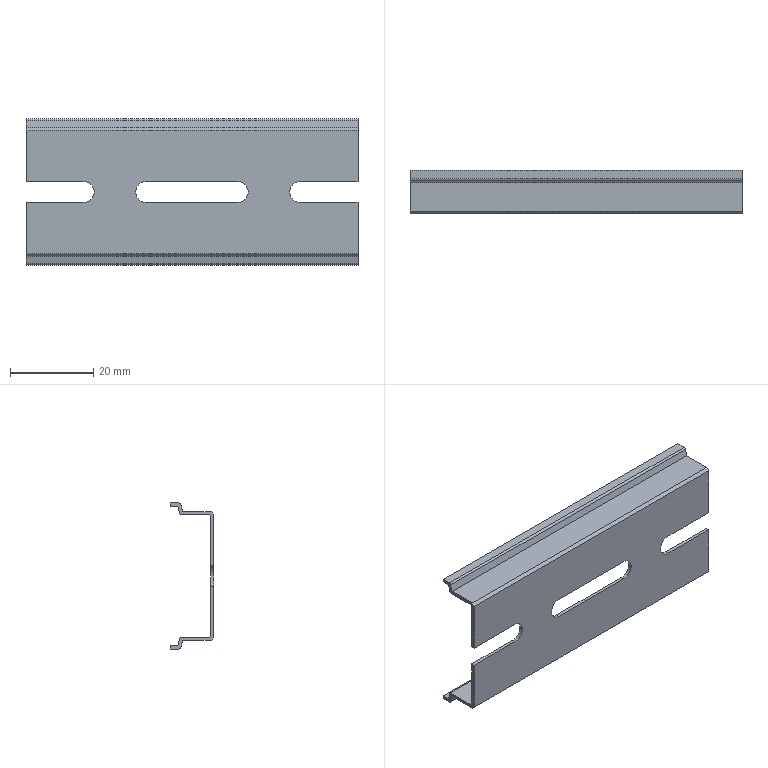Part | NX | 1 solid | 38 faces | box 79.8 x 10.5 x 35.1 mm | volume 3155 mm3 | plane 30 | cylinder 8 | commonest cylinder face diameters 5 x6 1 x2
STEP:
#1=CARTESIAN_POINT('',(44.9,-0.325,-0.15));
#2=VERTEX_POINT('',#1);
#3=CARTESIAN_POINT('',(44.9,-2.422,-0.15));
#4=VERTEX_POINT('',#3);
#5=CARTESIAN_POINT('',(44.9,0.,-0.15));
#6=DIRECTION('',(0.,-1.,0.));
#7=VECTOR('',#6,1000.);
#8=LINE('',#5,#7);
#9=EDGE_CURVE('',#2,#4,#8,.T.);
#10=ORIENTED_EDGE('',*,*,#9,.F.);
#11=CARTESIAN_POINT('',(-34.9,-0.325,-0.15));
#12=VERTEX_POINT('',#11);
#13=CARTESIAN_POINT('',(0.,-0.325,-0.15));
#14=DIRECTION('',(1.,0.,0.));
#15=VECTOR('',#14,1000.);
#16=LINE('',#13,#15);
#17=EDGE_CURVE('',#12,#2,#16,.T.);
#18=ORIENTED_EDGE('',*,*,#17,.F.);
#19=CARTESIAN_POINT('',(-34.9,-2.422,-0.15));
#20=VERTEX_POINT('',#19);
#21=CARTESIAN_POINT('',(-34.9,0.,-0.15));
#22=DIRECTION('',(0.,-1.,0.));
#23=VECTOR('',#22,1000.);
#24=LINE('',#21,#23);
#25=EDGE_CURVE('',#12,#20,#24,.T.);
#26=ORIENTED_EDGE('',*,*,#25,.T.);
#27=CARTESIAN_POINT('',(4.9,-2.422,-0.15));
#28=DIRECTION('',(-1.,0.,0.));
#29=VECTOR('',#28,1000.);
#30=LINE('',#27,#29);
#31=EDGE_CURVE('',#4,#20,#30,.T.);
#32=ORIENTED_EDGE('',*,*,#31,.F.);
#33=EDGE_LOOP('',(#10,#18,#26,#32));
#34=FACE_BOUND('',#33,.T.);
#35=CARTESIAN_POINT('',(4.9,-2.422,-0.15));
#36=DIRECTION('',(0.,0.,-1.));
#37=DIRECTION('',(0.,-1.,0.));
#38=AXIS2_PLACEMENT_3D('',#35,#36,#37);
#39=PLANE('',#38);
#40=ADVANCED_FACE('',(#34),#39,.F.);
#41=CARTESIAN_POINT('',(44.9,-10.169,-33.2));
#42=VERTEX_POINT('',#41);
#43=CARTESIAN_POINT('',(44.9,-3.325,-33.2));
#44=VERTEX_POINT('',#43);
#45=CARTESIAN_POINT('',(44.9,0.,-33.2));
#46=DIRECTION('',(0.,1.,0.));
#47=VECTOR('',#46,1000.);
#48=LINE('',#45,#47);
#49=EDGE_CURVE('',#42,#44,#48,.T.);
#50=ORIENTED_EDGE('',*,*,#49,.T.);
#51=CARTESIAN_POINT('',(44.9,-2.907,-34.871));
#52=VERTEX_POINT('',#51);
#53=CARTESIAN_POINT('',(44.9,-11.625,0.));
#54=DIRECTION('',(0.,0.2425,-0.9701));
#55=VECTOR('',#54,1000.);
#56=LINE('',#53,#55);
#57=EDGE_CURVE('',#44,#52,#56,.T.);
#58=ORIENTED_EDGE('',*,*,#57,.T.);
#59=CARTESIAN_POINT('',(44.9,-2.422,-35.25));
#60=VERTEX_POINT('',#59);
#61=CARTESIAN_POINT('',(44.9,-2.422,-34.75));
#62=DIRECTION('',(-1.,0.,0.));
#63=DIRECTION('',(0.,0.,1.));
#64=AXIS2_PLACEMENT_3D('',#61,#62,#63);
#65=CIRCLE('',#64,0.5);
#66=EDGE_CURVE('',#60,#52,#65,.T.);
#67=ORIENTED_EDGE('',*,*,#66,.F.);
#68=CARTESIAN_POINT('',(44.9,-0.325,-35.25));
#69=VERTEX_POINT('',#68);
#70=CARTESIAN_POINT('',(44.9,0.,-35.25));
#71=DIRECTION('',(0.,1.,0.));
#72=VECTOR('',#71,1000.);
#73=LINE('',#70,#72);
#74=EDGE_CURVE('',#60,#69,#73,.T.);
#75=ORIENTED_EDGE('',*,*,#74,.T.);
#76=CARTESIAN_POINT('',(44.9,-0.325,-34.45));
#77=VERTEX_POINT('',#76);
#78=CARTESIAN_POINT('',(44.9,-0.325,0.));
#79=DIRECTION('',(0.,0.,1.));
#80=VECTOR('',#79,1000.);
#81=LINE('',#78,#80);
#82=EDGE_CURVE('',#69,#77,#81,.T.);
#83=ORIENTED_EDGE('',*,*,#82,.T.);
#84=CARTESIAN_POINT('',(44.9,-2.188,-34.45));
#85=VERTEX_POINT('',#84);
#86=CARTESIAN_POINT('',(44.9,0.,-34.45));
#87=DIRECTION('',(0.,-1.,0.));
#88=VECTOR('',#87,1000.);
#89=LINE('',#86,#88);
#90=EDGE_CURVE('',#77,#85,#89,.T.);
#91=ORIENTED_EDGE('',*,*,#90,.T.);
#92=CARTESIAN_POINT('',(44.9,-2.7,-32.4));
#93=VERTEX_POINT('',#92);
#94=CARTESIAN_POINT('',(44.9,-10.8,0.));
#95=DIRECTION('',(0.,-0.2425,0.9701));
#96=VECTOR('',#95,1000.);
#97=LINE('',#94,#96);
#98=EDGE_CURVE('',#85,#93,#97,.T.);
#99=ORIENTED_EDGE('',*,*,#98,.T.);
#100=CARTESIAN_POINT('',(44.9,-9.834,-32.4));
#101=VERTEX_POINT('',#100);
#102=CARTESIAN_POINT('',(44.9,0.,-32.4));
#103=DIRECTION('',(0.,-1.,0.));
#104=VECTOR('',#103,1000.);
#105=LINE('',#102,#104);
#106=EDGE_CURVE('',#93,#101,#105,.T.);
#107=ORIENTED_EDGE('',*,*,#106,.T.);
#108=CARTESIAN_POINT('',(44.9,-10.025,-32.205));
#109=VERTEX_POINT('',#108);
#110=CARTESIAN_POINT('',(44.9,-41.673,0.));
#111=DIRECTION('',(0.,-0.7009,0.7133));
#112=VECTOR('',#111,1000.);
#113=LINE('',#110,#112);
#114=EDGE_CURVE('',#101,#109,#113,.T.);
#115=ORIENTED_EDGE('',*,*,#114,.T.);
#116=CARTESIAN_POINT('',(44.9,-10.025,-20.2));
#117=VERTEX_POINT('',#116);
#118=CARTESIAN_POINT('',(44.9,-10.025,0.));
#119=DIRECTION('',(0.,0.,1.));
#120=VECTOR('',#119,1000.);
#121=LINE('',#118,#120);
#122=EDGE_CURVE('',#109,#117,#121,.T.);
#123=ORIENTED_EDGE('',*,*,#122,.T.);
#124=CARTESIAN_POINT('',(44.9,-10.825,-20.2));
#125=VERTEX_POINT('',#124);
#126=CARTESIAN_POINT('',(44.9,0.,-20.2));
#127=DIRECTION('',(0.,-1.,0.));
#128=VECTOR('',#127,1000.);
#129=LINE('',#126,#128);
#130=EDGE_CURVE('',#117,#125,#129,.T.);
#131=ORIENTED_EDGE('',*,*,#130,.T.);
#132=CARTESIAN_POINT('',(44.9,-10.825,-32.532));
#133=VERTEX_POINT('',#132);
#134=CARTESIAN_POINT('',(44.9,-10.825,0.));
#135=DIRECTION('',(0.,0.,-1.));
#136=VECTOR('',#135,1000.);
#137=LINE('',#134,#136);
#138=EDGE_CURVE('',#125,#133,#137,.T.);
#139=ORIENTED_EDGE('',*,*,#138,.T.);
#140=CARTESIAN_POINT('',(44.9,-42.795,0.));
#141=DIRECTION('',(0.,0.7009,-0.7133));
#142=VECTOR('',#141,1000.);
#143=LINE('',#140,#142);
#144=EDGE_CURVE('',#133,#42,#143,.T.);
#145=ORIENTED_EDGE('',*,*,#144,.T.);
#146=EDGE_LOOP('',(#50,#58,#67,#75,#83,#91,#99,#107,#115,#123,#131,#139,#145));
#147=FACE_BOUND('',#146,.T.);
#148=CARTESIAN_POINT('',(44.9,-2.422,-0.65));
#149=DIRECTION('',(1.,0.,0.));
#150=DIRECTION('',(0.,0.,1.));
#151=AXIS2_PLACEMENT_3D('',#148,#149,#150);
#152=PLANE('',#151);
#153=ADVANCED_FACE('',(#147),#152,.T.);
#154=CARTESIAN_POINT('',(-34.9,-10.169,-33.2));
#155=VERTEX_POINT('',#154);
#156=CARTESIAN_POINT('',(-34.9,-3.325,-33.2));
#157=VERTEX_POINT('',#156);
#158=CARTESIAN_POINT('',(-34.9,0.,-33.2));
#159=DIRECTION('',(0.,1.,0.));
#160=VECTOR('',#159,1000.);
#161=LINE('',#158,#160);
#162=EDGE_CURVE('',#155,#157,#161,.T.);
#163=ORIENTED_EDGE('',*,*,#162,.T.);
#164=CARTESIAN_POINT('',(0.,-3.325,-33.2));
#165=DIRECTION('',(-1.,0.,0.));
#166=VECTOR('',#165,1000.);
#167=LINE('',#164,#166);
#168=EDGE_CURVE('',#44,#157,#167,.T.);
#169=ORIENTED_EDGE('',*,*,#168,.F.);
#170=ORIENTED_EDGE('',*,*,#49,.F.);
#171=CARTESIAN_POINT('',(0.,-10.169,-33.2));
#172=DIRECTION('',(-1.,0.,0.));
#173=VECTOR('',#172,1000.);
#174=LINE('',#171,#173);
#175=EDGE_CURVE('',#42,#155,#174,.T.);
#176=ORIENTED_EDGE('',*,*,#175,.T.);
#177=EDGE_LOOP('',(#163,#169,#170,#176));
#178=FACE_BOUND('',#177,.T.);
#179=CARTESIAN_POINT('',(4.9,-10.169,-33.2));
#180=DIRECTION('',(0.,0.,1.));
#181=DIRECTION('',(0.,-1.,0.));
#182=AXIS2_PLACEMENT_3D('',#179,#180,#181);
#183=PLANE('',#182);
#184=ADVANCED_FACE('',(#178),#183,.F.);
#185=ORIENTED_EDGE('',*,*,#138,.F.);
#186=CARTESIAN_POINT('',(31.,-10.825,-20.2));
#187=VERTEX_POINT('',#186);
#188=CARTESIAN_POINT('',(0.,-10.825,-20.2));
#189=DIRECTION('',(-1.,0.,0.));
#190=VECTOR('',#189,1000.);
#191=LINE('',#188,#190);
#192=EDGE_CURVE('',#125,#187,#191,.T.);
#193=ORIENTED_EDGE('',*,*,#192,.T.);
#194=CARTESIAN_POINT('',(28.5,-10.825,-17.7));
#195=VERTEX_POINT('',#194);
#196=CARTESIAN_POINT('',(31.,-10.825,-17.7));
#197=DIRECTION('',(0.,1.,0.));
#198=DIRECTION('',(-1.,0.,0.));
#199=AXIS2_PLACEMENT_3D('',#196,#197,#198);
#200=CIRCLE('',#199,2.5);
#201=EDGE_CURVE('',#187,#195,#200,.T.);
#202=ORIENTED_EDGE('',*,*,#201,.T.);
#203=CARTESIAN_POINT('',(31.,-10.825,-15.2));
#204=VERTEX_POINT('',#203);
#205=CARTESIAN_POINT('',(31.,-10.825,-17.7));
#206=DIRECTION('',(0.,1.,0.));
#207=DIRECTION('',(-1.,0.,0.));
#208=AXIS2_PLACEMENT_3D('',#205,#206,#207);
#209=CIRCLE('',#208,2.5);
#210=EDGE_CURVE('',#195,#204,#209,.T.);
#211=ORIENTED_EDGE('',*,*,#210,.T.);
#212=CARTESIAN_POINT('',(44.9,-10.825,-15.2));
#213=VERTEX_POINT('',#212);
#214=CARTESIAN_POINT('',(0.,-10.825,-15.2));
#215=DIRECTION('',(1.,0.,0.));
#216=VECTOR('',#215,1000.);
#217=LINE('',#214,#216);
#218=EDGE_CURVE('',#204,#213,#217,.T.);
#219=ORIENTED_EDGE('',*,*,#218,.T.);
#220=CARTESIAN_POINT('',(44.9,-10.825,-2.868));
#221=VERTEX_POINT('',#220);
#222=CARTESIAN_POINT('',(44.9,-10.825,0.));
#223=DIRECTION('',(0.,0.,-1.));
#224=VECTOR('',#223,1000.);
#225=LINE('',#222,#224);
#226=EDGE_CURVE('',#221,#213,#225,.T.);
#227=ORIENTED_EDGE('',*,*,#226,.F.);
#228=CARTESIAN_POINT('',(-34.9,-10.825,-2.868));
#229=VERTEX_POINT('',#228);
#230=CARTESIAN_POINT('',(0.,-10.825,-2.868));
#231=DIRECTION('',(1.,0.,0.));
#232=VECTOR('',#231,1000.);
#233=LINE('',#230,#232);
#234=EDGE_CURVE('',#229,#221,#233,.T.);
#235=ORIENTED_EDGE('',*,*,#234,.F.);
#236=CARTESIAN_POINT('',(-34.9,-10.825,-15.2));
#237=VERTEX_POINT('',#236);
#238=CARTESIAN_POINT('',(-34.9,-10.825,0.));
#239=DIRECTION('',(0.,0.,-1.));
#240=VECTOR('',#239,1000.);
#241=LINE('',#238,#240);
#242=EDGE_CURVE('',#229,#237,#241,.T.);
#243=ORIENTED_EDGE('',*,*,#242,.T.);
#244=CARTESIAN_POINT('',(-21.,-10.825,-15.2));
#245=VERTEX_POINT('',#244);
#246=CARTESIAN_POINT('',(0.,-10.825,-15.2));
#247=DIRECTION('',(1.,0.,0.));
#248=VECTOR('',#247,1000.);
#249=LINE('',#246,#248);
#250=EDGE_CURVE('',#237,#245,#249,.T.);
#251=ORIENTED_EDGE('',*,*,#250,.T.);
#252=CARTESIAN_POINT('',(-21.,-10.825,-20.2));
#253=VERTEX_POINT('',#252);
#254=CARTESIAN_POINT('',(-21.,-10.825,-17.7));
#255=DIRECTION('',(0.,1.,0.));
#256=DIRECTION('',(-1.,0.,0.));
#257=AXIS2_PLACEMENT_3D('',#254,#255,#256);
#258=CIRCLE('',#257,2.5);
#259=EDGE_CURVE('',#245,#253,#258,.T.);
#260=ORIENTED_EDGE('',*,*,#259,.T.);
#261=CARTESIAN_POINT('',(-34.9,-10.825,-20.2));
#262=VERTEX_POINT('',#261);
#263=CARTESIAN_POINT('',(0.,-10.825,-20.2));
#264=DIRECTION('',(-1.,0.,0.));
#265=VECTOR('',#264,1000.);
#266=LINE('',#263,#265);
#267=EDGE_CURVE('',#253,#262,#266,.T.);
#268=ORIENTED_EDGE('',*,*,#267,.T.);
#269=CARTESIAN_POINT('',(-34.9,-10.825,-32.532));
#270=VERTEX_POINT('',#269);
#271=CARTESIAN_POINT('',(-34.9,-10.825,0.));
#272=DIRECTION('',(0.,0.,-1.));
#273=VECTOR('',#272,1000.);
#274=LINE('',#271,#273);
#275=EDGE_CURVE('',#262,#270,#274,.T.);
#276=ORIENTED_EDGE('',*,*,#275,.T.);
#277=CARTESIAN_POINT('',(0.,-10.825,-32.532));
#278=DIRECTION('',(-1.,0.,0.));
#279=VECTOR('',#278,1000.);
#280=LINE('',#277,#279);
#281=EDGE_CURVE('',#133,#270,#280,.T.);
#282=ORIENTED_EDGE('',*,*,#281,.F.);
#283=EDGE_LOOP('',(#185,#193,#202,#211,#219,#227,#235,#243,#251,#260,#268,#276,#282));
#284=FACE_BOUND('',#283,.T.);
#285=CARTESIAN_POINT('',(16.,-10.825,-20.2));
#286=VERTEX_POINT('',#285);
#287=CARTESIAN_POINT('',(-6.,-10.825,-20.2));
#288=VERTEX_POINT('',#287);
#289=CARTESIAN_POINT('',(0.,-10.825,-20.2));
#290=DIRECTION('',(-1.,0.,0.));
#291=VECTOR('',#290,1000.);
#292=LINE('',#289,#291);
#293=EDGE_CURVE('',#286,#288,#292,.T.);
#294=ORIENTED_EDGE('',*,*,#293,.T.);
#295=CARTESIAN_POINT('',(-8.5,-10.825,-17.7));
#296=VERTEX_POINT('',#295);
#297=CARTESIAN_POINT('',(-6.,-10.825,-17.7));
#298=DIRECTION('',(0.,1.,0.));
#299=DIRECTION('',(-1.,0.,0.));
#300=AXIS2_PLACEMENT_3D('',#297,#298,#299);
#301=CIRCLE('',#300,2.5);
#302=EDGE_CURVE('',#288,#296,#301,.T.);
#303=ORIENTED_EDGE('',*,*,#302,.T.);
#304=CARTESIAN_POINT('',(-6.,-10.825,-15.2));
#305=VERTEX_POINT('',#304);
#306=CARTESIAN_POINT('',(-6.,-10.825,-17.7));
#307=DIRECTION('',(0.,1.,0.));
#308=DIRECTION('',(-1.,0.,0.));
#309=AXIS2_PLACEMENT_3D('',#306,#307,#308);
#310=CIRCLE('',#309,2.5);
#311=EDGE_CURVE('',#296,#305,#310,.T.);
#312=ORIENTED_EDGE('',*,*,#311,.T.);
#313=CARTESIAN_POINT('',(16.,-10.825,-15.2));
#314=VERTEX_POINT('',#313);
#315=CARTESIAN_POINT('',(0.,-10.825,-15.2));
#316=DIRECTION('',(1.,0.,0.));
#317=VECTOR('',#316,1000.);
#318=LINE('',#315,#317);
#319=EDGE_CURVE('',#305,#314,#318,.T.);
#320=ORIENTED_EDGE('',*,*,#319,.T.);
#321=CARTESIAN_POINT('',(16.,-10.825,-17.7));
#322=DIRECTION('',(0.,1.,0.));
#323=DIRECTION('',(-1.,0.,0.));
#324=AXIS2_PLACEMENT_3D('',#321,#322,#323);
#325=CIRCLE('',#324,2.5);
#326=EDGE_CURVE('',#314,#286,#325,.T.);
#327=ORIENTED_EDGE('',*,*,#326,.T.);
#328=EDGE_LOOP('',(#294,#303,#312,#320,#327));
#329=FACE_BOUND('',#328,.T.);
#330=CARTESIAN_POINT('',(4.9,-10.825,-2.868));
#331=DIRECTION('',(0.,1.,0.));
#332=DIRECTION('',(0.,0.,-1.));
#333=AXIS2_PLACEMENT_3D('',#330,#331,#332);
#334=PLANE('',#333);
#335=ADVANCED_FACE('',(#284,#329),#334,.F.);
#336=CARTESIAN_POINT('',(-34.9,-2.422,-35.25));
#337=VERTEX_POINT('',#336);
#338=CARTESIAN_POINT('',(-34.9,-2.907,-34.871));
#339=VERTEX_POINT('',#338);
#340=CARTESIAN_POINT('',(-34.9,-2.422,-34.75));
#341=DIRECTION('',(-1.,0.,0.));
#342=DIRECTION('',(0.,0.,1.));
#343=AXIS2_PLACEMENT_3D('',#340,#341,#342);
#344=CIRCLE('',#343,0.5);
#345=EDGE_CURVE('',#337,#339,#344,.T.);
#346=ORIENTED_EDGE('',*,*,#345,.F.);
#347=CARTESIAN_POINT('',(4.9,-2.422,-35.25));
#348=DIRECTION('',(1.,0.,0.));
#349=VECTOR('',#348,1000.);
#350=LINE('',#347,#349);
#351=EDGE_CURVE('',#337,#60,#350,.T.);
#352=ORIENTED_EDGE('',*,*,#351,.T.);
#353=ORIENTED_EDGE('',*,*,#66,.T.);
#354=CARTESIAN_POINT('',(4.9,-2.907,-34.871));
#355=DIRECTION('',(-1.,0.,0.));
#356=VECTOR('',#355,1000.);
#357=LINE('',#354,#356);
#358=EDGE_CURVE('',#52,#339,#357,.T.);
#359=ORIENTED_EDGE('',*,*,#358,.T.);
#360=EDGE_LOOP('',(#346,#352,#353,#359));
#361=FACE_BOUND('',#360,.T.);
#362=CARTESIAN_POINT('',(4.9,-2.422,-34.75));
#363=DIRECTION('',(-1.,0.,0.));
#364=DIRECTION('',(0.,0.,1.));
#365=AXIS2_PLACEMENT_3D('',#362,#363,#364);
#366=CYLINDRICAL_SURFACE('',#365,0.5);
#367=ADVANCED_FACE('',(#361),#366,.T.);
#368=CARTESIAN_POINT('',(-34.9,-0.325,-34.45));
#369=VERTEX_POINT('',#368);
#370=CARTESIAN_POINT('',(0.,-0.325,-34.45));
#371=DIRECTION('',(1.,0.,0.));
#372=VECTOR('',#371,1000.);
#373=LINE('',#370,#372);
#374=EDGE_CURVE('',#369,#77,#373,.T.);
#375=ORIENTED_EDGE('',*,*,#374,.T.);
#376=ORIENTED_EDGE('',*,*,#82,.F.);
#377=CARTESIAN_POINT('',(-34.9,-0.325,-35.25));
#378=VERTEX_POINT('',#377);
#379=CARTESIAN_POINT('',(0.,-0.325,-35.25));
#380=DIRECTION('',(1.,0.,0.));
#381=VECTOR('',#380,1000.);
#382=LINE('',#379,#381);
#383=EDGE_CURVE('',#378,#69,#382,.T.);
#384=ORIENTED_EDGE('',*,*,#383,.F.);
#385=CARTESIAN_POINT('',(-34.9,-0.325,0.));
#386=DIRECTION('',(0.,0.,1.));
#387=VECTOR('',#386,1000.);
#388=LINE('',#385,#387);
#389=EDGE_CURVE('',#378,#369,#388,.T.);
#390=ORIENTED_EDGE('',*,*,#389,.T.);
#391=EDGE_LOOP('',(#375,#376,#384,#390));
#392=FACE_BOUND('',#391,.T.);
#393=CARTESIAN_POINT('',(4.9,-0.325,-35.25));
#394=DIRECTION('',(0.,-1.,0.));
#395=DIRECTION('',(-1.,0.,0.));
#396=AXIS2_PLACEMENT_3D('',#393,#394,#395);
#397=PLANE('',#396);
#398=ADVANCED_FACE('',(#392),#397,.F.);
#399=CARTESIAN_POINT('',(-34.9,-3.325,-2.2));
#400=VERTEX_POINT('',#399);
#401=CARTESIAN_POINT('',(-34.9,-10.169,-2.2));
#402=VERTEX_POINT('',#401);
#403=CARTESIAN_POINT('',(-34.9,0.,-2.2));
#404=DIRECTION('',(0.,-1.,0.));
#405=VECTOR('',#404,1000.);
#406=LINE('',#403,#405);
#407=EDGE_CURVE('',#400,#402,#406,.T.);
#408=ORIENTED_EDGE('',*,*,#407,.T.);
#409=CARTESIAN_POINT('',(44.9,-10.169,-2.2));
#410=VERTEX_POINT('',#409);
#411=CARTESIAN_POINT('',(0.,-10.169,-2.2));
#412=DIRECTION('',(1.,0.,0.));
#413=VECTOR('',#412,1000.);
#414=LINE('',#411,#413);
#415=EDGE_CURVE('',#402,#410,#414,.T.);
#416=ORIENTED_EDGE('',*,*,#415,.T.);
#417=CARTESIAN_POINT('',(44.9,-3.325,-2.2));
#418=VERTEX_POINT('',#417);
#419=CARTESIAN_POINT('',(44.9,0.,-2.2));
#420=DIRECTION('',(0.,-1.,0.));
#421=VECTOR('',#420,1000.);
#422=LINE('',#419,#421);
#423=EDGE_CURVE('',#418,#410,#422,.T.);
#424=ORIENTED_EDGE('',*,*,#423,.F.);
#425=CARTESIAN_POINT('',(0.,-3.325,-2.2));
#426=DIRECTION('',(1.,0.,0.));
#427=VECTOR('',#426,1000.);
#428=LINE('',#425,#427);
#429=EDGE_CURVE('',#400,#418,#428,.T.);
#430=ORIENTED_EDGE('',*,*,#429,.F.);
#431=EDGE_LOOP('',(#408,#416,#424,#430));
#432=FACE_BOUND('',#431,.T.);
#433=CARTESIAN_POINT('',(4.9,-3.325,-2.2));
#434=DIRECTION('',(0.,0.,-1.));
#435=DIRECTION('',(-1.,0.,0.));
#436=AXIS2_PLACEMENT_3D('',#433,#434,#435);
#437=PLANE('',#436);
#438=ADVANCED_FACE('',(#432),#437,.F.);
#439=CARTESIAN_POINT('',(44.9,-0.325,-0.95));
#440=VERTEX_POINT('',#439);
#441=CARTESIAN_POINT('',(44.9,-0.325,0.));
#442=DIRECTION('',(0.,0.,1.));
#443=VECTOR('',#442,1000.);
#444=LINE('',#441,#443);
#445=EDGE_CURVE('',#440,#2,#444,.T.);
#446=ORIENTED_EDGE('',*,*,#445,.F.);
#447=CARTESIAN_POINT('',(-34.9,-0.325,-0.95));
#448=VERTEX_POINT('',#447);
#449=CARTESIAN_POINT('',(0.,-0.325,-0.95));
#450=DIRECTION('',(-1.,0.,0.));
#451=VECTOR('',#450,1000.);
#452=LINE('',#449,#451);
#453=EDGE_CURVE('',#440,#448,#452,.T.);
#454=ORIENTED_EDGE('',*,*,#453,.T.);
#455=CARTESIAN_POINT('',(-34.9,-0.325,0.));
#456=DIRECTION('',(0.,0.,1.));
#457=VECTOR('',#456,1000.);
#458=LINE('',#455,#457);
#459=EDGE_CURVE('',#448,#12,#458,.T.);
#460=ORIENTED_EDGE('',*,*,#459,.T.);
#461=ORIENTED_EDGE('',*,*,#17,.T.);
#462=EDGE_LOOP('',(#446,#454,#460,#461));
#463=FACE_BOUND('',#462,.T.);
#464=CARTESIAN_POINT('',(4.9,-0.325,-3.9));
#465=DIRECTION('',(0.,-1.,0.));
#466=DIRECTION('',(-1.,0.,0.));
#467=AXIS2_PLACEMENT_3D('',#464,#465,#466);
#468=PLANE('',#467);
#469=ADVANCED_FACE('',(#463),#468,.F.);
#470=CARTESIAN_POINT('',(-34.9,-2.907,-0.5287));
#471=VERTEX_POINT('',#470);
#472=CARTESIAN_POINT('',(-34.9,-2.422,-0.65));
#473=DIRECTION('',(-1.,0.,0.));
#474=DIRECTION('',(0.,0.,1.));
#475=AXIS2_PLACEMENT_3D('',#472,#473,#474);
#476=CIRCLE('',#475,0.5);
#477=EDGE_CURVE('',#471,#20,#476,.T.);
#478=ORIENTED_EDGE('',*,*,#477,.F.);
#479=CARTESIAN_POINT('',(44.9,-2.907,-0.5287));
#480=VERTEX_POINT('',#479);
#481=CARTESIAN_POINT('',(4.9,-2.907,-0.5287));
#482=DIRECTION('',(1.,0.,0.));
#483=VECTOR('',#482,1000.);
#484=LINE('',#481,#483);
#485=EDGE_CURVE('',#471,#480,#484,.T.);
#486=ORIENTED_EDGE('',*,*,#485,.T.);
#487=CARTESIAN_POINT('',(44.9,-2.422,-0.65));
#488=DIRECTION('',(-1.,0.,0.));
#489=DIRECTION('',(0.,0.,1.));
#490=AXIS2_PLACEMENT_3D('',#487,#488,#489);
#491=CIRCLE('',#490,0.5);
#492=EDGE_CURVE('',#480,#4,#491,.T.);
#493=ORIENTED_EDGE('',*,*,#492,.T.);
#494=ORIENTED_EDGE('',*,*,#31,.T.);
#495=EDGE_LOOP('',(#478,#486,#493,#494));
#496=FACE_BOUND('',#495,.T.);
#497=CARTESIAN_POINT('',(4.9,-2.422,-0.65));
#498=DIRECTION('',(-1.,0.,0.));
#499=DIRECTION('',(0.,0.,1.));
#500=AXIS2_PLACEMENT_3D('',#497,#498,#499);
#501=CYLINDRICAL_SURFACE('',#500,0.5);
#502=ADVANCED_FACE('',(#496),#501,.T.);
#503=ORIENTED_EDGE('',*,*,#162,.F.);
#504=CARTESIAN_POINT('',(-34.9,-42.795,0.));
#505=DIRECTION('',(0.,0.7009,-0.7133));
#506=VECTOR('',#505,1000.);
#507=LINE('',#504,#506);
#508=EDGE_CURVE('',#270,#155,#507,.T.);
#509=ORIENTED_EDGE('',*,*,#508,.F.);
#510=ORIENTED_EDGE('',*,*,#275,.F.);
#511=CARTESIAN_POINT('',(-34.9,-10.025,-20.2));
#512=VERTEX_POINT('',#511);
#513=CARTESIAN_POINT('',(-34.9,0.,-20.2));
#514=DIRECTION('',(0.,-1.,0.));
#515=VECTOR('',#514,1000.);
#516=LINE('',#513,#515);
#517=EDGE_CURVE('',#512,#262,#516,.T.);
#518=ORIENTED_EDGE('',*,*,#517,.F.);
#519=CARTESIAN_POINT('',(-34.9,-10.025,-32.205));
#520=VERTEX_POINT('',#519);
#521=CARTESIAN_POINT('',(-34.9,-10.025,0.));
#522=DIRECTION('',(0.,0.,1.));
#523=VECTOR('',#522,1000.);
#524=LINE('',#521,#523);
#525=EDGE_CURVE('',#520,#512,#524,.T.);
#526=ORIENTED_EDGE('',*,*,#525,.F.);
#527=CARTESIAN_POINT('',(-34.9,-9.834,-32.4));
#528=VERTEX_POINT('',#527);
#529=CARTESIAN_POINT('',(-34.9,-41.673,0.));
#530=DIRECTION('',(0.,-0.7009,0.7133));
#531=VECTOR('',#530,1000.);
#532=LINE('',#529,#531);
#533=EDGE_CURVE('',#528,#520,#532,.T.);
#534=ORIENTED_EDGE('',*,*,#533,.F.);
#535=CARTESIAN_POINT('',(-34.9,-2.7,-32.4));
#536=VERTEX_POINT('',#535);
#537=CARTESIAN_POINT('',(-34.9,0.,-32.4));
#538=DIRECTION('',(0.,-1.,0.));
#539=VECTOR('',#538,1000.);
#540=LINE('',#537,#539);
#541=EDGE_CURVE('',#536,#528,#540,.T.);
#542=ORIENTED_EDGE('',*,*,#541,.F.);
#543=CARTESIAN_POINT('',(-34.9,-2.188,-34.45));
#544=VERTEX_POINT('',#543);
#545=CARTESIAN_POINT('',(-34.9,-10.8,0.));
#546=DIRECTION('',(0.,-0.2425,0.9701));
#547=VECTOR('',#546,1000.);
#548=LINE('',#545,#547);
#549=EDGE_CURVE('',#544,#536,#548,.T.);
#550=ORIENTED_EDGE('',*,*,#549,.F.);
#551=CARTESIAN_POINT('',(-34.9,0.,-34.45));
#552=DIRECTION('',(0.,-1.,0.));
#553=VECTOR('',#552,1000.);
#554=LINE('',#551,#553);
#555=EDGE_CURVE('',#369,#544,#554,.T.);
#556=ORIENTED_EDGE('',*,*,#555,.F.);
#557=ORIENTED_EDGE('',*,*,#389,.F.);
#558=CARTESIAN_POINT('',(-34.9,0.,-35.25));
#559=DIRECTION('',(0.,1.,0.));
#560=VECTOR('',#559,1000.);
#561=LINE('',#558,#560);
#562=EDGE_CURVE('',#337,#378,#561,.T.);
#563=ORIENTED_EDGE('',*,*,#562,.F.);
#564=ORIENTED_EDGE('',*,*,#345,.T.);
#565=CARTESIAN_POINT('',(-34.9,-11.625,0.));
#566=DIRECTION('',(0.,0.2425,-0.9701));
#567=VECTOR('',#566,1000.);
#568=LINE('',#565,#567);
#569=EDGE_CURVE('',#157,#339,#568,.T.);
#570=ORIENTED_EDGE('',*,*,#569,.F.);
#571=EDGE_LOOP('',(#503,#509,#510,#518,#526,#534,#542,#550,#556,#557,#563,#564,#570));
#572=FACE_BOUND('',#571,.T.);
#573=CARTESIAN_POINT('',(-34.9,-2.422,-0.65));
#574=DIRECTION('',(1.,0.,0.));
#575=DIRECTION('',(0.,0.,1.));
#576=AXIS2_PLACEMENT_3D('',#573,#574,#575);
#577=PLANE('',#576);
#578=ADVANCED_FACE('',(#572),#577,.F.);
#579=CARTESIAN_POINT('',(44.9,-8.007,0.));
#580=DIRECTION('',(0.,-0.7009,-0.7133));
#581=VECTOR('',#580,1000.);
#582=LINE('',#579,#581);
#583=EDGE_CURVE('',#410,#221,#582,.T.);
#584=ORIENTED_EDGE('',*,*,#583,.F.);
#585=ORIENTED_EDGE('',*,*,#415,.F.);
#586=CARTESIAN_POINT('',(-34.9,-8.007,0.));
#587=DIRECTION('',(0.,-0.7009,-0.7133));
#588=VECTOR('',#587,1000.);
#589=LINE('',#586,#588);
#590=EDGE_CURVE('',#402,#229,#589,.T.);
#591=ORIENTED_EDGE('',*,*,#590,.T.);
#592=ORIENTED_EDGE('',*,*,#234,.T.);
#593=EDGE_LOOP('',(#584,#585,#591,#592));
#594=FACE_BOUND('',#593,.T.);
#595=CARTESIAN_POINT('',(4.9,-10.825,-2.868));
#596=DIRECTION('',(0.,0.7133,-0.7009));
#597=DIRECTION('',(-1.,0.,0.));
#598=AXIS2_PLACEMENT_3D('',#595,#596,#597);
#599=PLANE('',#598);
#600=ADVANCED_FACE('',(#594),#599,.F.);
#601=ORIENTED_EDGE('',*,*,#74,.F.);
#602=ORIENTED_EDGE('',*,*,#351,.F.);
#603=ORIENTED_EDGE('',*,*,#562,.T.);
#604=ORIENTED_EDGE('',*,*,#383,.T.);
#605=EDGE_LOOP('',(#601,#602,#603,#604));
#606=FACE_BOUND('',#605,.T.);
#607=CARTESIAN_POINT('',(4.9,-2.422,-35.25));
#608=DIRECTION('',(0.,0.,1.));
#609=DIRECTION('',(0.,-1.,0.));
#610=AXIS2_PLACEMENT_3D('',#607,#608,#609);
#611=PLANE('',#610);
#612=ADVANCED_FACE('',(#606),#611,.F.);
#613=ORIENTED_EDGE('',*,*,#144,.F.);
#614=ORIENTED_EDGE('',*,*,#281,.T.);
#615=ORIENTED_EDGE('',*,*,#508,.T.);
#616=ORIENTED_EDGE('',*,*,#175,.F.);
#617=EDGE_LOOP('',(#613,#614,#615,#616));
#618=FACE_BOUND('',#617,.T.);
#619=CARTESIAN_POINT('',(4.9,-10.825,-32.532));
#620=DIRECTION('',(0.,0.7133,0.7009));
#621=DIRECTION('',(1.,0.,0.));
#622=AXIS2_PLACEMENT_3D('',#619,#620,#621);
#623=PLANE('',#622);
#624=ADVANCED_FACE('',(#618),#623,.F.);
#625=ORIENTED_EDGE('',*,*,#57,.F.);
#626=ORIENTED_EDGE('',*,*,#168,.T.);
#627=ORIENTED_EDGE('',*,*,#569,.T.);
#628=ORIENTED_EDGE('',*,*,#358,.F.);
#629=EDGE_LOOP('',(#625,#626,#627,#628));
#630=FACE_BOUND('',#629,.T.);
#631=CARTESIAN_POINT('',(4.9,-2.907,-34.871));
#632=DIRECTION('',(0.,0.9701,0.2425));
#633=DIRECTION('',(1.,0.,0.));
#634=AXIS2_PLACEMENT_3D('',#631,#632,#633);
#635=PLANE('',#634);
#636=ADVANCED_FACE('',(#630),#635,.F.);
#637=CARTESIAN_POINT('',(44.9,-2.775,0.));
#638=DIRECTION('',(0.,-0.2425,-0.9701));
#639=VECTOR('',#638,1000.);
#640=LINE('',#637,#639);
#641=EDGE_CURVE('',#480,#418,#640,.T.);
#642=ORIENTED_EDGE('',*,*,#641,.F.);
#643=ORIENTED_EDGE('',*,*,#485,.F.);
#644=CARTESIAN_POINT('',(-34.9,-2.775,0.));
#645=DIRECTION('',(0.,-0.2425,-0.9701));
#646=VECTOR('',#645,1000.);
#647=LINE('',#644,#646);
#648=EDGE_CURVE('',#471,#400,#647,.T.);
#649=ORIENTED_EDGE('',*,*,#648,.T.);
#650=ORIENTED_EDGE('',*,*,#429,.T.);
#651=EDGE_LOOP('',(#642,#643,#649,#650));
#652=FACE_BOUND('',#651,.T.);
#653=CARTESIAN_POINT('',(4.9,-2.907,-0.5287));
#654=DIRECTION('',(0.,0.9701,-0.2425));
#655=DIRECTION('',(-1.,0.,0.));
#656=AXIS2_PLACEMENT_3D('',#653,#654,#655);
#657=PLANE('',#656);
#658=ADVANCED_FACE('',(#652),#657,.F.);
#659=ORIENTED_EDGE('',*,*,#549,.T.);
#660=CARTESIAN_POINT('',(0.,-2.7,-32.4));
#661=DIRECTION('',(-1.,0.,0.));
#662=VECTOR('',#661,1000.);
#663=LINE('',#660,#662);
#664=EDGE_CURVE('',#93,#536,#663,.T.);
#665=ORIENTED_EDGE('',*,*,#664,.F.);
#666=ORIENTED_EDGE('',*,*,#98,.F.);
#667=CARTESIAN_POINT('',(0.,-2.188,-34.45));
#668=DIRECTION('',(-1.,0.,0.));
#669=VECTOR('',#668,1000.);
#670=LINE('',#667,#669);
#671=EDGE_CURVE('',#85,#544,#670,.T.);
#672=ORIENTED_EDGE('',*,*,#671,.T.);
#673=EDGE_LOOP('',(#659,#665,#666,#672));
#674=FACE_BOUND('',#673,.T.);
#675=CARTESIAN_POINT('',(5.88,-2.7,-32.4));
#676=DIRECTION('',(0.,-0.9701,-0.2425));
#677=DIRECTION('',(0.,0.2425,-0.9701));
#678=AXIS2_PLACEMENT_3D('',#675,#676,#677);
#679=PLANE('',#678);
#680=ADVANCED_FACE('',(#674),#679,.F.);
#681=ORIENTED_EDGE('',*,*,#106,.F.);
#682=ORIENTED_EDGE('',*,*,#664,.T.);
#683=ORIENTED_EDGE('',*,*,#541,.T.);
#684=CARTESIAN_POINT('',(0.,-9.834,-32.4));
#685=DIRECTION('',(-1.,0.,0.));
#686=VECTOR('',#685,1000.);
#687=LINE('',#684,#686);
#688=EDGE_CURVE('',#101,#528,#687,.T.);
#689=ORIENTED_EDGE('',*,*,#688,.F.);
#690=EDGE_LOOP('',(#681,#682,#683,#689));
#691=FACE_BOUND('',#690,.T.);
#692=CARTESIAN_POINT('',(5.88,-9.834,-32.4));
#693=DIRECTION('',(0.,0.,-1.));
#694=DIRECTION('',(0.,-1.,0.));
#695=AXIS2_PLACEMENT_3D('',#692,#693,#694);
#696=PLANE('',#695);
#697=ADVANCED_FACE('',(#691),#696,.F.);
#698=ORIENTED_EDGE('',*,*,#114,.F.);
#699=ORIENTED_EDGE('',*,*,#688,.T.);
#700=ORIENTED_EDGE('',*,*,#533,.T.);
#701=CARTESIAN_POINT('',(0.,-10.025,-32.205));
#702=DIRECTION('',(-1.,0.,0.));
#703=VECTOR('',#702,1000.);
#704=LINE('',#701,#703);
#705=EDGE_CURVE('',#109,#520,#704,.T.);
#706=ORIENTED_EDGE('',*,*,#705,.F.);
#707=EDGE_LOOP('',(#698,#699,#700,#706));
#708=FACE_BOUND('',#707,.T.);
#709=CARTESIAN_POINT('',(5.88,-10.025,-32.205));
#710=DIRECTION('',(0.,-0.7133,-0.7009));
#711=DIRECTION('',(0.,0.7009,-0.7133));
#712=AXIS2_PLACEMENT_3D('',#709,#710,#711);
#713=PLANE('',#712);
#714=ADVANCED_FACE('',(#708),#713,.F.);
#715=CARTESIAN_POINT('',(-34.9,-10.025,-15.2));
#716=VERTEX_POINT('',#715);
#717=CARTESIAN_POINT('',(-34.9,-10.025,-3.195));
#718=VERTEX_POINT('',#717);
#719=CARTESIAN_POINT('',(-34.9,-10.025,0.));
#720=DIRECTION('',(0.,0.,1.));
#721=VECTOR('',#720,1000.);
#722=LINE('',#719,#721);
#723=EDGE_CURVE('',#716,#718,#722,.T.);
#724=ORIENTED_EDGE('',*,*,#723,.T.);
#725=CARTESIAN_POINT('',(44.9,-10.025,-3.195));
#726=VERTEX_POINT('',#725);
#727=CARTESIAN_POINT('',(0.,-10.025,-3.195));
#728=DIRECTION('',(-1.,0.,0.));
#729=VECTOR('',#728,1000.);
#730=LINE('',#727,#729);
#731=EDGE_CURVE('',#726,#718,#730,.T.);
#732=ORIENTED_EDGE('',*,*,#731,.F.);
#733=CARTESIAN_POINT('',(44.9,-10.025,-15.2));
#734=VERTEX_POINT('',#733);
#735=CARTESIAN_POINT('',(44.9,-10.025,0.));
#736=DIRECTION('',(0.,0.,1.));
#737=VECTOR('',#736,1000.);
#738=LINE('',#735,#737);
#739=EDGE_CURVE('',#734,#726,#738,.T.);
#740=ORIENTED_EDGE('',*,*,#739,.F.);
#741=CARTESIAN_POINT('',(31.,-10.025,-15.2));
#742=VERTEX_POINT('',#741);
#743=CARTESIAN_POINT('',(0.,-10.025,-15.2));
#744=DIRECTION('',(-1.,0.,0.));
#745=VECTOR('',#744,1000.);
#746=LINE('',#743,#745);
#747=EDGE_CURVE('',#734,#742,#746,.T.);
#748=ORIENTED_EDGE('',*,*,#747,.T.);
#749=CARTESIAN_POINT('',(28.5,-10.025,-17.7));
#750=VERTEX_POINT('',#749);
#751=CARTESIAN_POINT('',(31.,-10.025,-17.7));
#752=DIRECTION('',(0.,1.,0.));
#753=DIRECTION('',(-1.,0.,0.));
#754=AXIS2_PLACEMENT_3D('',#751,#752,#753);
#755=CIRCLE('',#754,2.5);
#756=EDGE_CURVE('',#750,#742,#755,.T.);
#757=ORIENTED_EDGE('',*,*,#756,.F.);
#758=CARTESIAN_POINT('',(31.,-10.025,-20.2));
#759=VERTEX_POINT('',#758);
#760=CARTESIAN_POINT('',(31.,-10.025,-17.7));
#761=DIRECTION('',(0.,1.,0.));
#762=DIRECTION('',(-1.,0.,0.));
#763=AXIS2_PLACEMENT_3D('',#760,#761,#762);
#764=CIRCLE('',#763,2.5);
#765=EDGE_CURVE('',#759,#750,#764,.T.);
#766=ORIENTED_EDGE('',*,*,#765,.F.);
#767=CARTESIAN_POINT('',(0.,-10.025,-20.2));
#768=DIRECTION('',(1.,0.,0.));
#769=VECTOR('',#768,1000.);
#770=LINE('',#767,#769);
#771=EDGE_CURVE('',#759,#117,#770,.T.);
#772=ORIENTED_EDGE('',*,*,#771,.T.);
#773=ORIENTED_EDGE('',*,*,#122,.F.);
#774=ORIENTED_EDGE('',*,*,#705,.T.);
#775=ORIENTED_EDGE('',*,*,#525,.T.);
#776=CARTESIAN_POINT('',(-21.,-10.025,-20.2));
#777=VERTEX_POINT('',#776);
#778=CARTESIAN_POINT('',(0.,-10.025,-20.2));
#779=DIRECTION('',(1.,0.,0.));
#780=VECTOR('',#779,1000.);
#781=LINE('',#778,#780);
#782=EDGE_CURVE('',#512,#777,#781,.T.);
#783=ORIENTED_EDGE('',*,*,#782,.T.);
#784=CARTESIAN_POINT('',(-21.,-10.025,-15.2));
#785=VERTEX_POINT('',#784);
#786=CARTESIAN_POINT('',(-21.,-10.025,-17.7));
#787=DIRECTION('',(0.,1.,0.));
#788=DIRECTION('',(-1.,0.,0.));
#789=AXIS2_PLACEMENT_3D('',#786,#787,#788);
#790=CIRCLE('',#789,2.5);
#791=EDGE_CURVE('',#785,#777,#790,.T.);
#792=ORIENTED_EDGE('',*,*,#791,.F.);
#793=CARTESIAN_POINT('',(0.,-10.025,-15.2));
#794=DIRECTION('',(-1.,0.,0.));
#795=VECTOR('',#794,1000.);
#796=LINE('',#793,#795);
#797=EDGE_CURVE('',#785,#716,#796,.T.);
#798=ORIENTED_EDGE('',*,*,#797,.T.);
#799=EDGE_LOOP('',(#724,#732,#740,#748,#757,#766,#772,#773,#774,#775,#783,#792,#798));
#800=FACE_BOUND('',#799,.T.);
#801=CARTESIAN_POINT('',(16.,-10.025,-15.2));
#802=VERTEX_POINT('',#801);
#803=CARTESIAN_POINT('',(-6.,-10.025,-15.2));
#804=VERTEX_POINT('',#803);
#805=CARTESIAN_POINT('',(0.,-10.025,-15.2));
#806=DIRECTION('',(-1.,0.,0.));
#807=VECTOR('',#806,1000.);
#808=LINE('',#805,#807);
#809=EDGE_CURVE('',#802,#804,#808,.T.);
#810=ORIENTED_EDGE('',*,*,#809,.T.);
#811=CARTESIAN_POINT('',(-8.5,-10.025,-17.7));
#812=VERTEX_POINT('',#811);
#813=CARTESIAN_POINT('',(-6.,-10.025,-17.7));
#814=DIRECTION('',(0.,1.,0.));
#815=DIRECTION('',(-1.,0.,0.));
#816=AXIS2_PLACEMENT_3D('',#813,#814,#815);
#817=CIRCLE('',#816,2.5);
#818=EDGE_CURVE('',#812,#804,#817,.T.);
#819=ORIENTED_EDGE('',*,*,#818,.F.);
#820=CARTESIAN_POINT('',(-6.,-10.025,-20.2));
#821=VERTEX_POINT('',#820);
#822=CARTESIAN_POINT('',(-6.,-10.025,-17.7));
#823=DIRECTION('',(0.,1.,0.));
#824=DIRECTION('',(-1.,0.,0.));
#825=AXIS2_PLACEMENT_3D('',#822,#823,#824);
#826=CIRCLE('',#825,2.5);
#827=EDGE_CURVE('',#821,#812,#826,.T.);
#828=ORIENTED_EDGE('',*,*,#827,.F.);
#829=CARTESIAN_POINT('',(16.,-10.025,-20.2));
#830=VERTEX_POINT('',#829);
#831=CARTESIAN_POINT('',(0.,-10.025,-20.2));
#832=DIRECTION('',(1.,0.,0.));
#833=VECTOR('',#832,1000.);
#834=LINE('',#831,#833);
#835=EDGE_CURVE('',#821,#830,#834,.T.);
#836=ORIENTED_EDGE('',*,*,#835,.T.);
#837=CARTESIAN_POINT('',(16.,-10.025,-17.7));
#838=DIRECTION('',(0.,1.,0.));
#839=DIRECTION('',(-1.,0.,0.));
#840=AXIS2_PLACEMENT_3D('',#837,#838,#839);
#841=CIRCLE('',#840,2.5);
#842=EDGE_CURVE('',#802,#830,#841,.T.);
#843=ORIENTED_EDGE('',*,*,#842,.F.);
#844=EDGE_LOOP('',(#810,#819,#828,#836,#843));
#845=FACE_BOUND('',#844,.T.);
#846=CARTESIAN_POINT('',(5.88,-10.025,-3.195));
#847=DIRECTION('',(0.,-1.,0.));
#848=DIRECTION('',(-1.,0.,0.));
#849=AXIS2_PLACEMENT_3D('',#846,#847,#848);
#850=PLANE('',#849);
#851=ADVANCED_FACE('',(#800,#845),#850,.F.);
#852=CARTESIAN_POINT('',(44.9,-9.834,-3.));
#853=VERTEX_POINT('',#852);
#854=CARTESIAN_POINT('',(44.9,-6.885,0.));
#855=DIRECTION('',(0.,0.7009,0.7133));
#856=VECTOR('',#855,1000.);
#857=LINE('',#854,#856);
#858=EDGE_CURVE('',#726,#853,#857,.T.);
#859=ORIENTED_EDGE('',*,*,#858,.F.);
#860=ORIENTED_EDGE('',*,*,#731,.T.);
#861=CARTESIAN_POINT('',(-34.9,-9.834,-3.));
#862=VERTEX_POINT('',#861);
#863=CARTESIAN_POINT('',(-34.9,-6.885,0.));
#864=DIRECTION('',(0.,0.7009,0.7133));
#865=VECTOR('',#864,1000.);
#866=LINE('',#863,#865);
#867=EDGE_CURVE('',#718,#862,#866,.T.);
#868=ORIENTED_EDGE('',*,*,#867,.T.);
#869=CARTESIAN_POINT('',(0.,-9.834,-3.));
#870=DIRECTION('',(-1.,0.,0.));
#871=VECTOR('',#870,1000.);
#872=LINE('',#869,#871);
#873=EDGE_CURVE('',#853,#862,#872,.T.);
#874=ORIENTED_EDGE('',*,*,#873,.F.);
#875=EDGE_LOOP('',(#859,#860,#868,#874));
#876=FACE_BOUND('',#875,.T.);
#877=CARTESIAN_POINT('',(5.88,-9.834,-3.));
#878=DIRECTION('',(0.,-0.7133,0.7009));
#879=DIRECTION('',(-1.,0.,0.));
#880=AXIS2_PLACEMENT_3D('',#877,#878,#879);
#881=PLANE('',#880);
#882=ADVANCED_FACE('',(#876),#881,.F.);
#883=CARTESIAN_POINT('',(-34.9,-2.7,-3.));
#884=VERTEX_POINT('',#883);
#885=CARTESIAN_POINT('',(-34.9,0.,-3.));
#886=DIRECTION('',(0.,1.,0.));
#887=VECTOR('',#886,1000.);
#888=LINE('',#885,#887);
#889=EDGE_CURVE('',#862,#884,#888,.T.);
#890=ORIENTED_EDGE('',*,*,#889,.T.);
#891=CARTESIAN_POINT('',(44.9,-2.7,-3.));
#892=VERTEX_POINT('',#891);
#893=CARTESIAN_POINT('',(0.,-2.7,-3.));
#894=DIRECTION('',(-1.,0.,0.));
#895=VECTOR('',#894,1000.);
#896=LINE('',#893,#895);
#897=EDGE_CURVE('',#892,#884,#896,.T.);
#898=ORIENTED_EDGE('',*,*,#897,.F.);
#899=CARTESIAN_POINT('',(44.9,0.,-3.));
#900=DIRECTION('',(0.,1.,0.));
#901=VECTOR('',#900,1000.);
#902=LINE('',#899,#901);
#903=EDGE_CURVE('',#853,#892,#902,.T.);
#904=ORIENTED_EDGE('',*,*,#903,.F.);
#905=ORIENTED_EDGE('',*,*,#873,.T.);
#906=EDGE_LOOP('',(#890,#898,#904,#905));
#907=FACE_BOUND('',#906,.T.);
#908=CARTESIAN_POINT('',(5.88,-2.7,-3.));
#909=DIRECTION('',(0.,0.,1.));
#910=DIRECTION('',(0.,-1.,0.));
#911=AXIS2_PLACEMENT_3D('',#908,#909,#910);
#912=PLANE('',#911);
#913=ADVANCED_FACE('',(#907),#912,.F.);
#914=CARTESIAN_POINT('',(44.9,-2.188,-0.95));
#915=VERTEX_POINT('',#914);
#916=CARTESIAN_POINT('',(44.9,-1.95,0.));
#917=DIRECTION('',(0.,0.2425,0.9701));
#918=VECTOR('',#917,1000.);
#919=LINE('',#916,#918);
#920=EDGE_CURVE('',#892,#915,#919,.T.);
#921=ORIENTED_EDGE('',*,*,#920,.F.);
#922=ORIENTED_EDGE('',*,*,#897,.T.);
#923=CARTESIAN_POINT('',(-34.9,-2.188,-0.95));
#924=VERTEX_POINT('',#923);
#925=CARTESIAN_POINT('',(-34.9,-1.95,0.));
#926=DIRECTION('',(0.,0.2425,0.9701));
#927=VECTOR('',#926,1000.);
#928=LINE('',#925,#927);
#929=EDGE_CURVE('',#884,#924,#928,.T.);
#930=ORIENTED_EDGE('',*,*,#929,.T.);
#931=CARTESIAN_POINT('',(0.,-2.188,-0.95));
#932=DIRECTION('',(-1.,0.,0.));
#933=VECTOR('',#932,1000.);
#934=LINE('',#931,#933);
#935=EDGE_CURVE('',#915,#924,#934,.T.);
#936=ORIENTED_EDGE('',*,*,#935,.F.);
#937=EDGE_LOOP('',(#921,#922,#930,#936));
#938=FACE_BOUND('',#937,.T.);
#939=CARTESIAN_POINT('',(5.88,-2.188,-0.95));
#940=DIRECTION('',(0.,-0.9701,0.2425));
#941=DIRECTION('',(-1.,0.,0.));
#942=AXIS2_PLACEMENT_3D('',#939,#940,#941);
#943=PLANE('',#942);
#944=ADVANCED_FACE('',(#938),#943,.F.);
#945=CARTESIAN_POINT('',(44.9,0.,-0.95));
#946=DIRECTION('',(0.,1.,0.));
#947=VECTOR('',#946,1000.);
#948=LINE('',#945,#947);
#949=EDGE_CURVE('',#915,#440,#948,.T.);
#950=ORIENTED_EDGE('',*,*,#949,.F.);
#951=ORIENTED_EDGE('',*,*,#935,.T.);
#952=CARTESIAN_POINT('',(-34.9,0.,-0.95));
#953=DIRECTION('',(0.,1.,0.));
#954=VECTOR('',#953,1000.);
#955=LINE('',#952,#954);
#956=EDGE_CURVE('',#924,#448,#955,.T.);
#957=ORIENTED_EDGE('',*,*,#956,.T.);
#958=ORIENTED_EDGE('',*,*,#453,.F.);
#959=EDGE_LOOP('',(#950,#951,#957,#958));
#960=FACE_BOUND('',#959,.T.);
#961=CARTESIAN_POINT('',(5.88,-0.325,-0.95));
#962=DIRECTION('',(0.,0.,1.));
#963=DIRECTION('',(0.,-1.,0.));
#964=AXIS2_PLACEMENT_3D('',#961,#962,#963);
#965=PLANE('',#964);
#966=ADVANCED_FACE('',(#960),#965,.F.);
#967=ORIENTED_EDGE('',*,*,#555,.T.);
#968=ORIENTED_EDGE('',*,*,#671,.F.);
#969=ORIENTED_EDGE('',*,*,#90,.F.);
#970=ORIENTED_EDGE('',*,*,#374,.F.);
#971=EDGE_LOOP('',(#967,#968,#969,#970));
#972=FACE_BOUND('',#971,.T.);
#973=CARTESIAN_POINT('',(5.88,-2.188,-34.45));
#974=DIRECTION('',(0.,0.,-1.));
#975=DIRECTION('',(0.,-1.,0.));
#976=AXIS2_PLACEMENT_3D('',#973,#974,#975);
#977=PLANE('',#976);
#978=ADVANCED_FACE('',(#972),#977,.F.);
#979=CARTESIAN_POINT('',(-34.9,0.,-15.2));
#980=DIRECTION('',(0.,1.,0.));
#981=VECTOR('',#980,1000.);
#982=LINE('',#979,#981);
#983=EDGE_CURVE('',#237,#716,#982,.T.);
#984=ORIENTED_EDGE('',*,*,#983,.F.);
#985=ORIENTED_EDGE('',*,*,#242,.F.);
#986=ORIENTED_EDGE('',*,*,#590,.F.);
#987=ORIENTED_EDGE('',*,*,#407,.F.);
#988=ORIENTED_EDGE('',*,*,#648,.F.);
#989=ORIENTED_EDGE('',*,*,#477,.T.);
#990=ORIENTED_EDGE('',*,*,#25,.F.);
#991=ORIENTED_EDGE('',*,*,#459,.F.);
#992=ORIENTED_EDGE('',*,*,#956,.F.);
#993=ORIENTED_EDGE('',*,*,#929,.F.);
#994=ORIENTED_EDGE('',*,*,#889,.F.);
#995=ORIENTED_EDGE('',*,*,#867,.F.);
#996=ORIENTED_EDGE('',*,*,#723,.F.);
#997=EDGE_LOOP('',(#984,#985,#986,#987,#988,#989,#990,#991,#992,#993,#994,#995,#996));
#998=FACE_BOUND('',#997,.T.);
#999=CARTESIAN_POINT('',(-34.9,-2.422,-0.65));
#1000=DIRECTION('',(1.,0.,0.));
#1001=DIRECTION('',(0.,0.,1.));
#1002=AXIS2_PLACEMENT_3D('',#999,#1000,#1001);
#1003=PLANE('',#1002);
#1004=ADVANCED_FACE('',(#998),#1003,.F.);
#1005=CARTESIAN_POINT('',(44.9,0.,-15.2));
#1006=DIRECTION('',(0.,1.,0.));
#1007=VECTOR('',#1006,1000.);
#1008=LINE('',#1005,#1007);
#1009=EDGE_CURVE('',#213,#734,#1008,.T.);
#1010=ORIENTED_EDGE('',*,*,#1009,.T.);
#1011=ORIENTED_EDGE('',*,*,#739,.T.);
#1012=ORIENTED_EDGE('',*,*,#858,.T.);
#1013=ORIENTED_EDGE('',*,*,#903,.T.);
#1014=ORIENTED_EDGE('',*,*,#920,.T.);
#1015=ORIENTED_EDGE('',*,*,#949,.T.);
#1016=ORIENTED_EDGE('',*,*,#445,.T.);
#1017=ORIENTED_EDGE('',*,*,#9,.T.);
#1018=ORIENTED_EDGE('',*,*,#492,.F.);
#1019=ORIENTED_EDGE('',*,*,#641,.T.);
#1020=ORIENTED_EDGE('',*,*,#423,.T.);
#1021=ORIENTED_EDGE('',*,*,#583,.T.);
#1022=ORIENTED_EDGE('',*,*,#226,.T.);
#1023=EDGE_LOOP('',(#1010,#1011,#1012,#1013,#1014,#1015,#1016,#1017,#1018,#1019,#1020,#1021,#1022));
#1024=FACE_BOUND('',#1023,.T.);
#1025=CARTESIAN_POINT('',(44.9,-2.422,-0.65));
#1026=DIRECTION('',(1.,0.,0.));
#1027=DIRECTION('',(0.,0.,1.));
#1028=AXIS2_PLACEMENT_3D('',#1025,#1026,#1027);
#1029=PLANE('',#1028);
#1030=ADVANCED_FACE('',(#1024),#1029,.T.);
#1031=ORIENTED_EDGE('',*,*,#250,.F.);
#1032=ORIENTED_EDGE('',*,*,#983,.T.);
#1033=ORIENTED_EDGE('',*,*,#797,.F.);
#1034=CARTESIAN_POINT('',(-21.,-11.875,-15.2));
#1035=DIRECTION('',(0.,1.,0.));
#1036=VECTOR('',#1035,1000.);
#1037=LINE('',#1034,#1036);
#1038=EDGE_CURVE('',#245,#785,#1037,.T.);
#1039=ORIENTED_EDGE('',*,*,#1038,.F.);
#1040=EDGE_LOOP('',(#1031,#1032,#1033,#1039));
#1041=FACE_BOUND('',#1040,.T.);
#1042=CARTESIAN_POINT('',(-21.,-11.875,-15.2));
#1043=DIRECTION('',(0.,0.,1.));
#1044=DIRECTION('',(0.,-1.,0.));
#1045=AXIS2_PLACEMENT_3D('',#1042,#1043,#1044);
#1046=PLANE('',#1045);
#1047=ADVANCED_FACE('',(#1041),#1046,.F.);
#1048=CARTESIAN_POINT('',(28.5,-11.875,-17.7));
#1049=DIRECTION('',(0.,1.,0.));
#1050=VECTOR('',#1049,1000.);
#1051=LINE('',#1048,#1050);
#1052=EDGE_CURVE('',#195,#750,#1051,.T.);
#1053=ORIENTED_EDGE('',*,*,#1052,.F.);
#1054=ORIENTED_EDGE('',*,*,#201,.F.);
#1055=CARTESIAN_POINT('',(31.,-11.875,-20.2));
#1056=DIRECTION('',(0.,1.,0.));
#1057=VECTOR('',#1056,1000.);
#1058=LINE('',#1055,#1057);
#1059=EDGE_CURVE('',#187,#759,#1058,.T.);
#1060=ORIENTED_EDGE('',*,*,#1059,.T.);
#1061=ORIENTED_EDGE('',*,*,#765,.T.);
#1062=EDGE_LOOP('',(#1053,#1054,#1060,#1061));
#1063=FACE_BOUND('',#1062,.T.);
#1064=CARTESIAN_POINT('',(31.,-11.875,-17.7));
#1065=DIRECTION('',(0.,1.,0.));
#1066=DIRECTION('',(-1.,0.,0.));
#1067=AXIS2_PLACEMENT_3D('',#1064,#1065,#1066);
#1068=CYLINDRICAL_SURFACE('',#1067,2.5);
#1069=ADVANCED_FACE('',(#1063),#1068,.F.);
#1070=ORIENTED_EDGE('',*,*,#771,.F.);
#1071=ORIENTED_EDGE('',*,*,#1059,.F.);
#1072=ORIENTED_EDGE('',*,*,#192,.F.);
#1073=ORIENTED_EDGE('',*,*,#130,.F.);
#1074=EDGE_LOOP('',(#1070,#1071,#1072,#1073));
#1075=FACE_BOUND('',#1074,.T.);
#1076=CARTESIAN_POINT('',(31.,-11.875,-20.2));
#1077=DIRECTION('',(0.,0.,-1.));
#1078=DIRECTION('',(0.,-1.,0.));
#1079=AXIS2_PLACEMENT_3D('',#1076,#1077,#1078);
#1080=PLANE('',#1079);
#1081=ADVANCED_FACE('',(#1075),#1080,.F.);
#1082=ORIENTED_EDGE('',*,*,#267,.F.);
#1083=CARTESIAN_POINT('',(-21.,-11.875,-20.2));
#1084=DIRECTION('',(0.,1.,0.));
#1085=VECTOR('',#1084,1000.);
#1086=LINE('',#1083,#1085);
#1087=EDGE_CURVE('',#253,#777,#1086,.T.);
#1088=ORIENTED_EDGE('',*,*,#1087,.T.);
#1089=ORIENTED_EDGE('',*,*,#782,.F.);
#1090=ORIENTED_EDGE('',*,*,#517,.T.);
#1091=EDGE_LOOP('',(#1082,#1088,#1089,#1090));
#1092=FACE_BOUND('',#1091,.T.);
#1093=CARTESIAN_POINT('',(-24.9,-11.875,-20.2));
#1094=DIRECTION('',(0.,0.,-1.));
#1095=DIRECTION('',(0.,-1.,0.));
#1096=AXIS2_PLACEMENT_3D('',#1093,#1094,#1095);
#1097=PLANE('',#1096);
#1098=ADVANCED_FACE('',(#1092),#1097,.F.);
#1099=ORIENTED_EDGE('',*,*,#809,.F.);
#1100=CARTESIAN_POINT('',(16.,-11.875,-15.2));
#1101=DIRECTION('',(0.,1.,0.));
#1102=VECTOR('',#1101,1000.);
#1103=LINE('',#1100,#1102);
#1104=EDGE_CURVE('',#314,#802,#1103,.T.);
#1105=ORIENTED_EDGE('',*,*,#1104,.F.);
#1106=ORIENTED_EDGE('',*,*,#319,.F.);
#1107=CARTESIAN_POINT('',(-6.,-11.875,-15.2));
#1108=DIRECTION('',(0.,1.,0.));
#1109=VECTOR('',#1108,1000.);
#1110=LINE('',#1107,#1109);
#1111=EDGE_CURVE('',#305,#804,#1110,.T.);
#1112=ORIENTED_EDGE('',*,*,#1111,.T.);
#1113=EDGE_LOOP('',(#1099,#1105,#1106,#1112));
#1114=FACE_BOUND('',#1113,.T.);
#1115=CARTESIAN_POINT('',(16.,-11.875,-15.2));
#1116=DIRECTION('',(0.,0.,1.));
#1117=DIRECTION('',(0.,-1.,0.));
#1118=AXIS2_PLACEMENT_3D('',#1115,#1116,#1117);
#1119=PLANE('',#1118);
#1120=ADVANCED_FACE('',(#1114),#1119,.F.);
#1121=ORIENTED_EDGE('',*,*,#326,.F.);
#1122=ORIENTED_EDGE('',*,*,#1104,.T.);
#1123=ORIENTED_EDGE('',*,*,#842,.T.);
#1124=CARTESIAN_POINT('',(16.,-11.875,-20.2));
#1125=DIRECTION('',(0.,1.,0.));
#1126=VECTOR('',#1125,1000.);
#1127=LINE('',#1124,#1126);
#1128=EDGE_CURVE('',#286,#830,#1127,.T.);
#1129=ORIENTED_EDGE('',*,*,#1128,.F.);
#1130=EDGE_LOOP('',(#1121,#1122,#1123,#1129));
#1131=FACE_BOUND('',#1130,.T.);
#1132=CARTESIAN_POINT('',(16.,-11.875,-17.7));
#1133=DIRECTION('',(0.,1.,0.));
#1134=DIRECTION('',(-1.,0.,0.));
#1135=AXIS2_PLACEMENT_3D('',#1132,#1133,#1134);
#1136=CYLINDRICAL_SURFACE('',#1135,2.5);
#1137=ADVANCED_FACE('',(#1131),#1136,.F.);
#1138=ORIENTED_EDGE('',*,*,#835,.F.);
#1139=CARTESIAN_POINT('',(-6.,-11.875,-20.2));
#1140=DIRECTION('',(0.,1.,0.));
#1141=VECTOR('',#1140,1000.);
#1142=LINE('',#1139,#1141);
#1143=EDGE_CURVE('',#288,#821,#1142,.T.);
#1144=ORIENTED_EDGE('',*,*,#1143,.F.);
#1145=ORIENTED_EDGE('',*,*,#293,.F.);
#1146=ORIENTED_EDGE('',*,*,#1128,.T.);
#1147=EDGE_LOOP('',(#1138,#1144,#1145,#1146));
#1148=FACE_BOUND('',#1147,.T.);
#1149=CARTESIAN_POINT('',(-6.,-11.875,-20.2));
#1150=DIRECTION('',(0.,0.,-1.));
#1151=DIRECTION('',(0.,-1.,0.));
#1152=AXIS2_PLACEMENT_3D('',#1149,#1150,#1151);
#1153=PLANE('',#1152);
#1154=ADVANCED_FACE('',(#1148),#1153,.F.);
#1155=CARTESIAN_POINT('',(-8.5,-11.875,-17.7));
#1156=DIRECTION('',(0.,1.,0.));
#1157=VECTOR('',#1156,1000.);
#1158=LINE('',#1155,#1157);
#1159=EDGE_CURVE('',#296,#812,#1158,.T.);
#1160=ORIENTED_EDGE('',*,*,#1159,.F.);
#1161=ORIENTED_EDGE('',*,*,#302,.F.);
#1162=ORIENTED_EDGE('',*,*,#1143,.T.);
#1163=ORIENTED_EDGE('',*,*,#827,.T.);
#1164=EDGE_LOOP('',(#1160,#1161,#1162,#1163));
#1165=FACE_BOUND('',#1164,.T.);
#1166=CARTESIAN_POINT('',(-6.,-11.875,-17.7));
#1167=DIRECTION('',(0.,1.,0.));
#1168=DIRECTION('',(-1.,0.,0.));
#1169=AXIS2_PLACEMENT_3D('',#1166,#1167,#1168);
#1170=CYLINDRICAL_SURFACE('',#1169,2.5);
#1171=ADVANCED_FACE('',(#1165),#1170,.F.);
#1172=ORIENTED_EDGE('',*,*,#747,.F.);
#1173=ORIENTED_EDGE('',*,*,#1009,.F.);
#1174=ORIENTED_EDGE('',*,*,#218,.F.);
#1175=CARTESIAN_POINT('',(31.,-11.875,-15.2));
#1176=DIRECTION('',(0.,1.,0.));
#1177=VECTOR('',#1176,1000.);
#1178=LINE('',#1175,#1177);
#1179=EDGE_CURVE('',#204,#742,#1178,.T.);
#1180=ORIENTED_EDGE('',*,*,#1179,.T.);
#1181=EDGE_LOOP('',(#1172,#1173,#1174,#1180));
#1182=FACE_BOUND('',#1181,.T.);
#1183=CARTESIAN_POINT('',(34.9,-11.875,-15.2));
#1184=DIRECTION('',(0.,0.,1.));
#1185=DIRECTION('',(0.,-1.,0.));
#1186=AXIS2_PLACEMENT_3D('',#1183,#1184,#1185);
#1187=PLANE('',#1186);
#1188=ADVANCED_FACE('',(#1182),#1187,.F.);
#1189=ORIENTED_EDGE('',*,*,#791,.T.);
#1190=ORIENTED_EDGE('',*,*,#1087,.F.);
#1191=ORIENTED_EDGE('',*,*,#259,.F.);
#1192=ORIENTED_EDGE('',*,*,#1038,.T.);
#1193=EDGE_LOOP('',(#1189,#1190,#1191,#1192));
#1194=FACE_BOUND('',#1193,.T.);
#1195=CARTESIAN_POINT('',(-21.,-11.875,-17.7));
#1196=DIRECTION('',(0.,1.,0.));
#1197=DIRECTION('',(-1.,0.,0.));
#1198=AXIS2_PLACEMENT_3D('',#1195,#1196,#1197);
#1199=CYLINDRICAL_SURFACE('',#1198,2.5);
#1200=ADVANCED_FACE('',(#1194),#1199,.F.);
#1201=ORIENTED_EDGE('',*,*,#311,.F.);
#1202=ORIENTED_EDGE('',*,*,#1159,.T.);
#1203=ORIENTED_EDGE('',*,*,#818,.T.);
#1204=ORIENTED_EDGE('',*,*,#1111,.F.);
#1205=EDGE_LOOP('',(#1201,#1202,#1203,#1204));
#1206=FACE_BOUND('',#1205,.T.);
#1207=CARTESIAN_POINT('',(-6.,-11.875,-17.7));
#1208=DIRECTION('',(0.,1.,0.));
#1209=DIRECTION('',(-1.,0.,0.));
#1210=AXIS2_PLACEMENT_3D('',#1207,#1208,#1209);
#1211=CYLINDRICAL_SURFACE('',#1210,2.5);
#1212=ADVANCED_FACE('',(#1206),#1211,.F.);
#1213=ORIENTED_EDGE('',*,*,#210,.F.);
#1214=ORIENTED_EDGE('',*,*,#1052,.T.);
#1215=ORIENTED_EDGE('',*,*,#756,.T.);
#1216=ORIENTED_EDGE('',*,*,#1179,.F.);
#1217=EDGE_LOOP('',(#1213,#1214,#1215,#1216));
#1218=FACE_BOUND('',#1217,.T.);
#1219=CARTESIAN_POINT('',(31.,-11.875,-17.7));
#1220=DIRECTION('',(0.,1.,0.));
#1221=DIRECTION('',(-1.,0.,0.));
#1222=AXIS2_PLACEMENT_3D('',#1219,#1220,#1221);
#1223=CYLINDRICAL_SURFACE('',#1222,2.5);
#1224=ADVANCED_FACE('',(#1218),#1223,.F.);
#1225=CLOSED_SHELL('',(#40,#153,#184,#335,#367,#398,#438,#469,#502,#578,#600,#612,#624,#636,#658,#680,#697,#714,#851,#882,#913,#944,#966,#978,#1004,#1030,#1047,#1069,#1081,#1098,#1120,#1137,#1154,#1171,#1188,#1200,#1212,#1224));
#1226=MANIFOLD_SOLID_BREP('',#1225);
#1227=(LENGTH_UNIT()NAMED_UNIT(*)SI_UNIT(.MILLI.,.METRE.));
#1228=UNCERTAINTY_MEASURE_WITH_UNIT(LENGTH_MEASURE(0.00001),#1227,'','');
#1229=(NAMED_UNIT(*)PLANE_ANGLE_UNIT()SI_UNIT($,.RADIAN.));
#1230=(NAMED_UNIT(*)SI_UNIT($,.STERADIAN.)SOLID_ANGLE_UNIT());
#1231=(GEOMETRIC_REPRESENTATION_CONTEXT(3)GLOBAL_UNCERTAINTY_ASSIGNED_CONTEXT((#1228))GLOBAL_UNIT_ASSIGNED_CONTEXT((#1227,#1229,#1230))REPRESENTATION_CONTEXT('',''));
#1232=ADVANCED_BREP_SHAPE_REPRESENTATION('',(#1226),#1231);